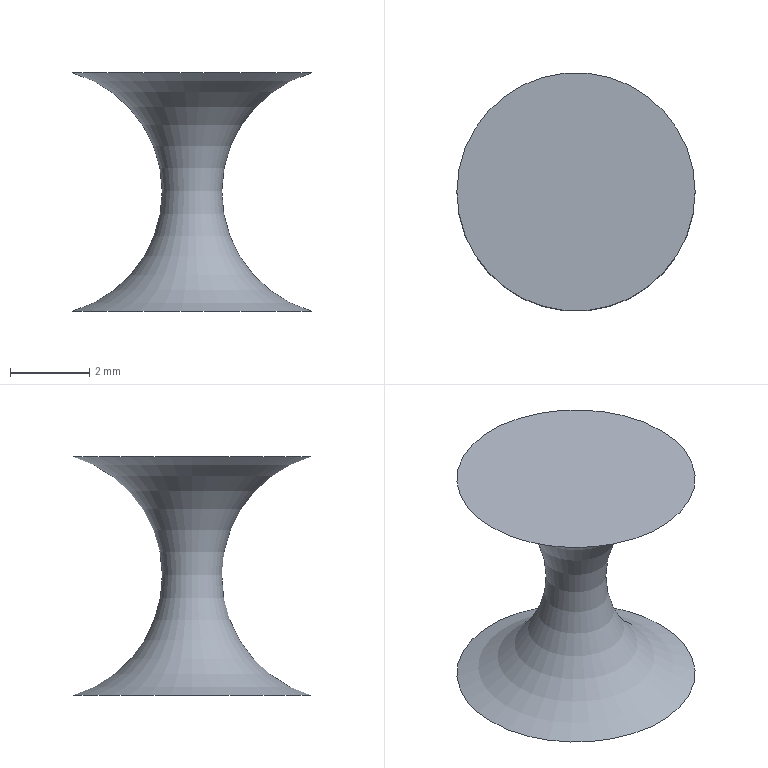Part | NX | features DATUM_CSYS 2, SKETCH 1, SWP104 1 | 1 solid | 3 faces | box 6 x 6 x 6 mm | volume 40.648 mm3 | plane 2 | torus 1
STEP:
#1=CARTESIAN_POINT('',(-3.,0.,0.));
#2=VERTEX_POINT('',#1);
#3=CARTESIAN_POINT('',(0.,0.,0.));
#4=DIRECTION('',(0.,0.,-1.));
#5=DIRECTION('',(-1.,0.,0.));
#6=AXIS2_PLACEMENT_3D('',#3,#4,#5);
#7=CIRCLE('',#6,3.);
#8=EDGE_CURVE('',#2,#2,#7,.T.);
#9=ORIENTED_EDGE('',*,*,#8,.T.);
#10=EDGE_LOOP('',(#9));
#11=FACE_BOUND('',#10,.T.);
#12=CARTESIAN_POINT('',(0.,0.,0.));
#13=DIRECTION('',(0.,0.,-1.));
#14=DIRECTION('',(-1.,0.,0.));
#15=AXIS2_PLACEMENT_3D('',#12,#13,#14);
#16=PLANE('',#15);
#17=ADVANCED_FACE('',(#11),#16,.T.);
#18=CARTESIAN_POINT('',(-3.,0.,6.));
#19=VERTEX_POINT('',#18);
#20=CARTESIAN_POINT('',(0.,0.,6.));
#21=DIRECTION('',(0.,0.,-1.));
#22=DIRECTION('',(-1.,0.,0.));
#23=AXIS2_PLACEMENT_3D('',#20,#21,#22);
#24=CIRCLE('',#23,3.);
#25=EDGE_CURVE('',#19,#19,#24,.T.);
#26=ORIENTED_EDGE('',*,*,#25,.T.);
#27=EDGE_LOOP('',(#26));
#28=FACE_BOUND('',#27,.T.);
#29=ORIENTED_EDGE('',*,*,#8,.F.);
#30=EDGE_LOOP('',(#29));
#31=FACE_BOUND('',#30,.T.);
#32=CARTESIAN_POINT('',(0.,0.,3.));
#33=DIRECTION('',(0.,0.,-1.));
#34=DIRECTION('',(-1.,0.,0.));
#35=AXIS2_PLACEMENT_3D('',#32,#33,#34);
#36=TOROIDAL_SURFACE('',#35,3.875,3.125);
#37=ADVANCED_FACE('',(#28,#31),#36,.F.);
#38=ORIENTED_EDGE('',*,*,#25,.F.);
#39=EDGE_LOOP('',(#38));
#40=FACE_BOUND('',#39,.T.);
#41=CARTESIAN_POINT('',(0.,3.,6.));
#42=DIRECTION('',(0.,0.,1.));
#43=DIRECTION('',(1.,0.,0.));
#44=AXIS2_PLACEMENT_3D('',#41,#42,#43);
#45=PLANE('',#44);
#46=ADVANCED_FACE('',(#40),#45,.T.);
#47=CLOSED_SHELL('',(#17,#37,#46));
#48=MANIFOLD_SOLID_BREP('',#47);
#49=(LENGTH_UNIT()NAMED_UNIT(*)SI_UNIT(.MILLI.,.METRE.));
#50=UNCERTAINTY_MEASURE_WITH_UNIT(LENGTH_MEASURE(0.00001),#49,'','');
#51=(NAMED_UNIT(*)PLANE_ANGLE_UNIT()SI_UNIT($,.RADIAN.));
#52=(NAMED_UNIT(*)SI_UNIT($,.STERADIAN.)SOLID_ANGLE_UNIT());
#53=(GEOMETRIC_REPRESENTATION_CONTEXT(3)GLOBAL_UNCERTAINTY_ASSIGNED_CONTEXT((#50))GLOBAL_UNIT_ASSIGNED_CONTEXT((#49,#51,#52))REPRESENTATION_CONTEXT('',''));
#54=ADVANCED_BREP_SHAPE_REPRESENTATION('',(#48),#53);